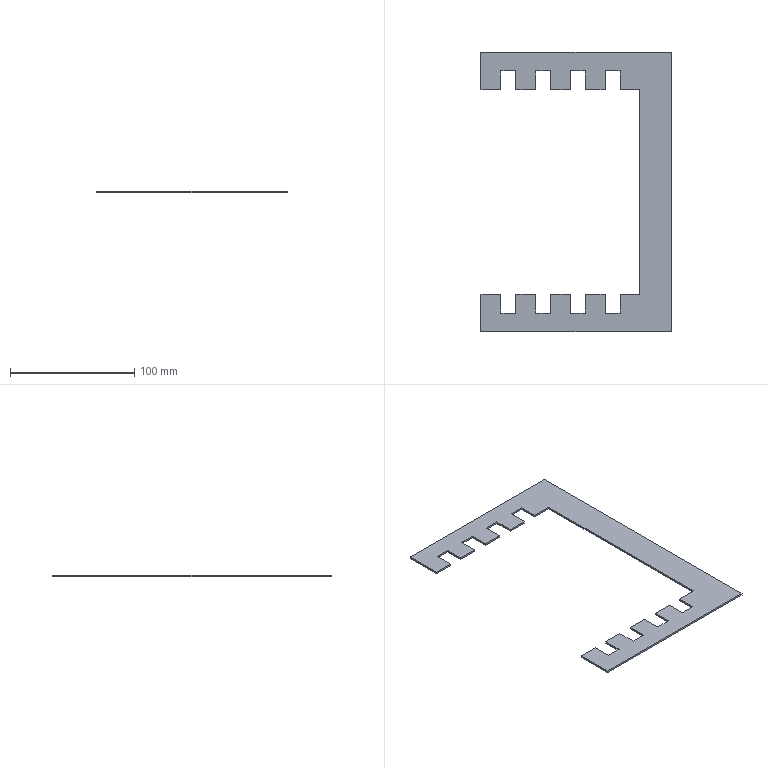Part | STEP file | A14-062 | 1 solid | 42 faces | box 153 x 225 x 1.5 mm | volume 17798 mm3 | plane 42